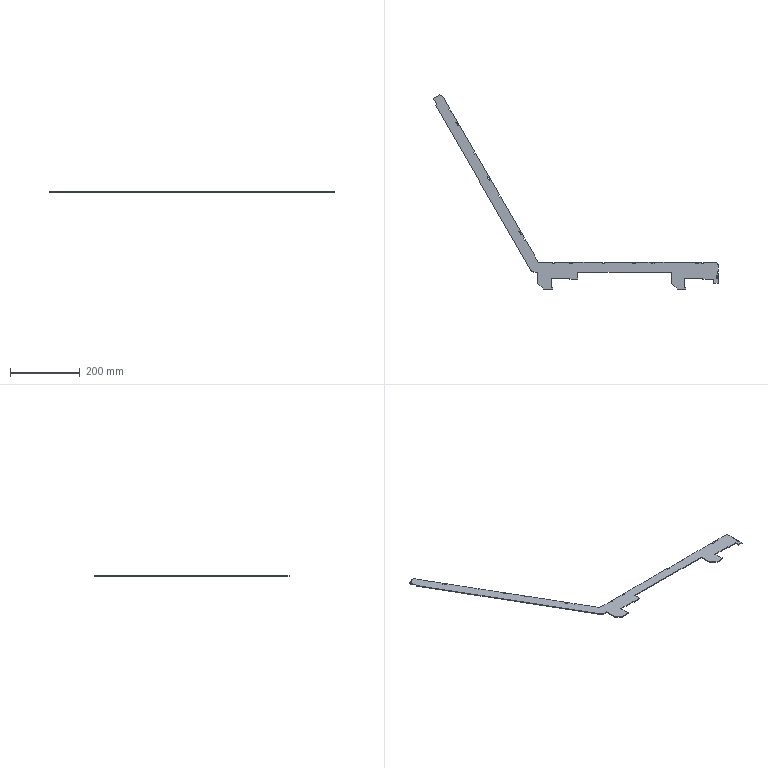Part | STEP file | zh003-1 | 1 solid | 104 faces | box 812.643 x 554.564 x 2 mm | volume 76512 mm3 | plane 100 | cylinder 4 | commonest cylinder face diameters 20 x3 8 x1